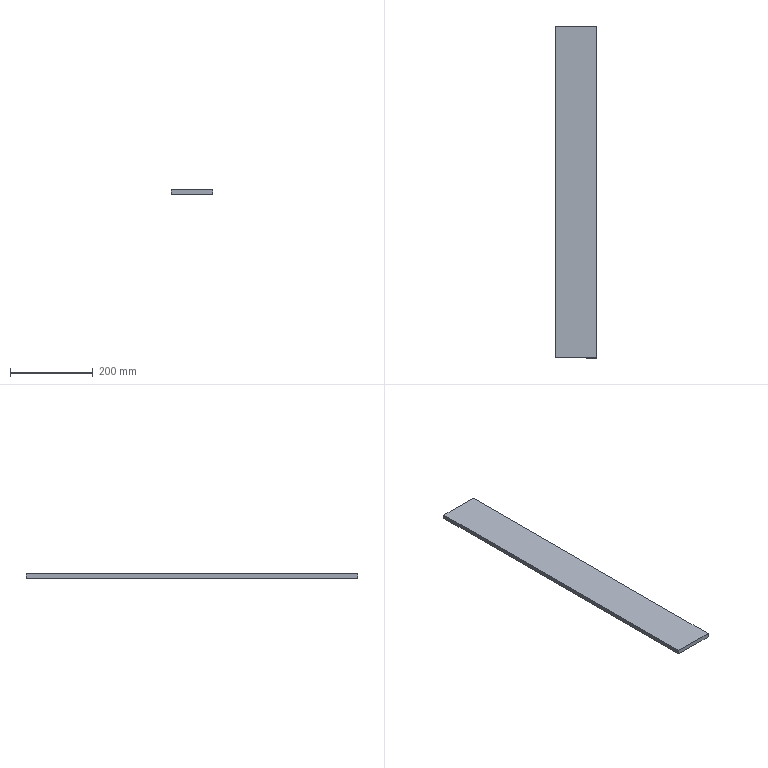Part | STEP file | C2 | 1 solid | 6 faces | box 100 x 800 x 10 mm | volume 800000 mm3 | plane 6
STEP:
#1=CARTESIAN_POINT('',(0.,0.,0.));
#2=DIRECTION('',(0.,0.,1.));
#3=DIRECTION('',(1.,0.,0.));
#4=AXIS2_PLACEMENT_3D('',#1,#2,#3);
#5=CARTESIAN_POINT('',(0.,800.,0.));
#6=VERTEX_POINT('',#5);
#7=CARTESIAN_POINT('',(0.,0.,0.));
#8=VERTEX_POINT('',#7);
#9=CARTESIAN_POINT('',(0.,800.,0.));
#10=DIRECTION('',(0.,-1.,0.));
#11=VECTOR('',#10,1.);
#12=LINE('',#9,#11);
#13=CARTESIAN_POINT('',(0.,800.,-10.));
#14=DIRECTION('',(-1.,0.,0.));
#15=DIRECTION('',(0.,-1.,0.));
#16=AXIS2_PLACEMENT_3D('',#13,#14,#15);
#17=PLANE('',#16);
#18=CARTESIAN_POINT('',(0.,10.));
#19=DIRECTION('',(1.,0.));
#20=VECTOR('',#19,1.);
#21=LINE('',#18,#20);
#22=(GEOMETRIC_REPRESENTATION_CONTEXT(2)PARAMETRIC_REPRESENTATION_CONTEXT()REPRESENTATION_CONTEXT('',''));
#23=DEFINITIONAL_REPRESENTATION('',(#21),#22);
#24=PCURVE('',#17,#23);
#25=CARTESIAN_POINT('',(0.,0.,0.));
#26=DIRECTION('',(0.,0.,1.));
#27=DIRECTION('',(1.,0.,0.));
#28=AXIS2_PLACEMENT_3D('',#25,#26,#27);
#29=PLANE('',#28);
#30=CARTESIAN_POINT('',(0.,800.));
#31=DIRECTION('',(0.,-1.));
#32=VECTOR('',#31,1.);
#33=LINE('',#30,#32);
#34=(GEOMETRIC_REPRESENTATION_CONTEXT(2)PARAMETRIC_REPRESENTATION_CONTEXT()REPRESENTATION_CONTEXT('',''));
#35=DEFINITIONAL_REPRESENTATION('',(#33),#34);
#36=PCURVE('',#29,#35);
#37=SURFACE_CURVE('',#12,(#24,#36),.PCURVE_S1.);
#38=EDGE_CURVE('',#6,#8,#37,.T.);
#39=ORIENTED_EDGE('',*,*,#38,.F.);
#40=CARTESIAN_POINT('',(0.,800.,-10.));
#41=VERTEX_POINT('',#40);
#42=CARTESIAN_POINT('',(0.,800.,-10.));
#43=DIRECTION('',(0.,0.,1.));
#44=VECTOR('',#43,1.);
#45=LINE('',#42,#44);
#46=CARTESIAN_POINT('',(0.,0.));
#47=DIRECTION('',(0.,1.));
#48=VECTOR('',#47,1.);
#49=LINE('',#46,#48);
#50=(GEOMETRIC_REPRESENTATION_CONTEXT(2)PARAMETRIC_REPRESENTATION_CONTEXT()REPRESENTATION_CONTEXT('',''));
#51=DEFINITIONAL_REPRESENTATION('',(#49),#50);
#52=PCURVE('',#17,#51);
#53=CARTESIAN_POINT('',(0.,800.,-10.));
#54=DIRECTION('',(0.,1.,0.));
#55=DIRECTION('',(-1.,0.,0.));
#56=AXIS2_PLACEMENT_3D('',#53,#54,#55);
#57=PLANE('',#56);
#58=CARTESIAN_POINT('',(0.,0.));
#59=DIRECTION('',(0.,1.));
#60=VECTOR('',#59,1.);
#61=LINE('',#58,#60);
#62=(GEOMETRIC_REPRESENTATION_CONTEXT(2)PARAMETRIC_REPRESENTATION_CONTEXT()REPRESENTATION_CONTEXT('',''));
#63=DEFINITIONAL_REPRESENTATION('',(#61),#62);
#64=PCURVE('',#57,#63);
#65=SURFACE_CURVE('',#45,(#52,#64),.PCURVE_S1.);
#66=EDGE_CURVE('',#41,#6,#65,.T.);
#67=ORIENTED_EDGE('',*,*,#66,.F.);
#68=CARTESIAN_POINT('',(0.,0.,-10.));
#69=VERTEX_POINT('',#68);
#70=CARTESIAN_POINT('',(0.,800.,-10.));
#71=DIRECTION('',(0.,-1.,0.));
#72=VECTOR('',#71,1.);
#73=LINE('',#70,#72);
#74=CARTESIAN_POINT('',(0.,0.));
#75=DIRECTION('',(1.,0.));
#76=VECTOR('',#75,1.);
#77=LINE('',#74,#76);
#78=(GEOMETRIC_REPRESENTATION_CONTEXT(2)PARAMETRIC_REPRESENTATION_CONTEXT()REPRESENTATION_CONTEXT('',''));
#79=DEFINITIONAL_REPRESENTATION('',(#77),#78);
#80=PCURVE('',#17,#79);
#81=CARTESIAN_POINT('',(0.,0.,-10.));
#82=DIRECTION('',(0.,0.,1.));
#83=DIRECTION('',(1.,0.,0.));
#84=AXIS2_PLACEMENT_3D('',#81,#82,#83);
#85=PLANE('',#84);
#86=CARTESIAN_POINT('',(0.,800.));
#87=DIRECTION('',(0.,-1.));
#88=VECTOR('',#87,1.);
#89=LINE('',#86,#88);
#90=(GEOMETRIC_REPRESENTATION_CONTEXT(2)PARAMETRIC_REPRESENTATION_CONTEXT()REPRESENTATION_CONTEXT('',''));
#91=DEFINITIONAL_REPRESENTATION('',(#89),#90);
#92=PCURVE('',#85,#91);
#93=SURFACE_CURVE('',#73,(#80,#92),.PCURVE_S1.);
#94=EDGE_CURVE('',#41,#69,#93,.T.);
#95=ORIENTED_EDGE('',*,*,#94,.T.);
#96=CARTESIAN_POINT('',(0.,0.,-10.));
#97=DIRECTION('',(0.,0.,1.));
#98=VECTOR('',#97,1.);
#99=LINE('',#96,#98);
#100=CARTESIAN_POINT('',(800.,0.));
#101=DIRECTION('',(0.,1.));
#102=VECTOR('',#101,1.);
#103=LINE('',#100,#102);
#104=(GEOMETRIC_REPRESENTATION_CONTEXT(2)PARAMETRIC_REPRESENTATION_CONTEXT()REPRESENTATION_CONTEXT('',''));
#105=DEFINITIONAL_REPRESENTATION('',(#103),#104);
#106=PCURVE('',#17,#105);
#107=CARTESIAN_POINT('',(0.,0.,-10.));
#108=DIRECTION('',(0.,-1.,0.));
#109=DIRECTION('',(1.,0.,0.));
#110=AXIS2_PLACEMENT_3D('',#107,#108,#109);
#111=PLANE('',#110);
#112=CARTESIAN_POINT('',(0.,0.));
#113=DIRECTION('',(0.,1.));
#114=VECTOR('',#113,1.);
#115=LINE('',#112,#114);
#116=(GEOMETRIC_REPRESENTATION_CONTEXT(2)PARAMETRIC_REPRESENTATION_CONTEXT()REPRESENTATION_CONTEXT('',''));
#117=DEFINITIONAL_REPRESENTATION('',(#115),#116);
#118=PCURVE('',#111,#117);
#119=SURFACE_CURVE('',#99,(#106,#118),.PCURVE_S1.);
#120=EDGE_CURVE('',#69,#8,#119,.T.);
#121=ORIENTED_EDGE('',*,*,#120,.T.);
#122=EDGE_LOOP('',(#39,#67,#95,#121));
#123=FACE_BOUND('',#122,.T.);
#124=ADVANCED_FACE('',(#123),#17,.T.);
#125=CARTESIAN_POINT('',(100.,800.,0.));
#126=VERTEX_POINT('',#125);
#127=CARTESIAN_POINT('',(0.,800.,0.));
#128=DIRECTION('',(-1.,0.,0.));
#129=VECTOR('',#128,1.);
#130=LINE('',#127,#129);
#131=CARTESIAN_POINT('',(0.,10.));
#132=DIRECTION('',(1.,0.));
#133=VECTOR('',#132,1.);
#134=LINE('',#131,#133);
#135=(GEOMETRIC_REPRESENTATION_CONTEXT(2)PARAMETRIC_REPRESENTATION_CONTEXT()REPRESENTATION_CONTEXT('',''));
#136=DEFINITIONAL_REPRESENTATION('',(#134),#135);
#137=PCURVE('',#57,#136);
#138=CARTESIAN_POINT('',(0.,800.));
#139=DIRECTION('',(-1.,0.));
#140=VECTOR('',#139,1.);
#141=LINE('',#138,#140);
#142=(GEOMETRIC_REPRESENTATION_CONTEXT(2)PARAMETRIC_REPRESENTATION_CONTEXT()REPRESENTATION_CONTEXT('',''));
#143=DEFINITIONAL_REPRESENTATION('',(#141),#142);
#144=PCURVE('',#29,#143);
#145=SURFACE_CURVE('',#130,(#137,#144),.PCURVE_S1.);
#146=EDGE_CURVE('',#126,#6,#145,.T.);
#147=ORIENTED_EDGE('',*,*,#146,.F.);
#148=CARTESIAN_POINT('',(100.,800.,-10.));
#149=VERTEX_POINT('',#148);
#150=CARTESIAN_POINT('',(100.,800.,-10.));
#151=DIRECTION('',(0.,0.,1.));
#152=VECTOR('',#151,1.);
#153=LINE('',#150,#152);
#154=CARTESIAN_POINT('',(-100.,0.));
#155=DIRECTION('',(0.,1.));
#156=VECTOR('',#155,1.);
#157=LINE('',#154,#156);
#158=(GEOMETRIC_REPRESENTATION_CONTEXT(2)PARAMETRIC_REPRESENTATION_CONTEXT()REPRESENTATION_CONTEXT('',''));
#159=DEFINITIONAL_REPRESENTATION('',(#157),#158);
#160=PCURVE('',#57,#159);
#161=CARTESIAN_POINT('',(100.,800.,-10.));
#162=DIRECTION('',(1.,0.,0.));
#163=DIRECTION('',(0.,1.,0.));
#164=AXIS2_PLACEMENT_3D('',#161,#162,#163);
#165=PLANE('',#164);
#166=CARTESIAN_POINT('',(0.,0.));
#167=DIRECTION('',(0.,1.));
#168=VECTOR('',#167,1.);
#169=LINE('',#166,#168);
#170=(GEOMETRIC_REPRESENTATION_CONTEXT(2)PARAMETRIC_REPRESENTATION_CONTEXT()REPRESENTATION_CONTEXT('',''));
#171=DEFINITIONAL_REPRESENTATION('',(#169),#170);
#172=PCURVE('',#165,#171);
#173=SURFACE_CURVE('',#153,(#160,#172),.PCURVE_S1.);
#174=EDGE_CURVE('',#149,#126,#173,.T.);
#175=ORIENTED_EDGE('',*,*,#174,.F.);
#176=CARTESIAN_POINT('',(0.,800.,-10.));
#177=DIRECTION('',(-1.,0.,0.));
#178=VECTOR('',#177,1.);
#179=LINE('',#176,#178);
#180=CARTESIAN_POINT('',(0.,0.));
#181=DIRECTION('',(1.,0.));
#182=VECTOR('',#181,1.);
#183=LINE('',#180,#182);
#184=(GEOMETRIC_REPRESENTATION_CONTEXT(2)PARAMETRIC_REPRESENTATION_CONTEXT()REPRESENTATION_CONTEXT('',''));
#185=DEFINITIONAL_REPRESENTATION('',(#183),#184);
#186=PCURVE('',#57,#185);
#187=CARTESIAN_POINT('',(0.,800.));
#188=DIRECTION('',(-1.,0.));
#189=VECTOR('',#188,1.);
#190=LINE('',#187,#189);
#191=(GEOMETRIC_REPRESENTATION_CONTEXT(2)PARAMETRIC_REPRESENTATION_CONTEXT()REPRESENTATION_CONTEXT('',''));
#192=DEFINITIONAL_REPRESENTATION('',(#190),#191);
#193=PCURVE('',#85,#192);
#194=SURFACE_CURVE('',#179,(#186,#193),.PCURVE_S1.);
#195=EDGE_CURVE('',#149,#41,#194,.T.);
#196=ORIENTED_EDGE('',*,*,#195,.T.);
#197=ORIENTED_EDGE('',*,*,#66,.T.);
#198=EDGE_LOOP('',(#147,#175,#196,#197));
#199=FACE_BOUND('',#198,.T.);
#200=ADVANCED_FACE('',(#199),#57,.T.);
#201=CARTESIAN_POINT('',(100.,0.,0.));
#202=VERTEX_POINT('',#201);
#203=CARTESIAN_POINT('',(100.,800.,0.));
#204=DIRECTION('',(0.,1.,0.));
#205=VECTOR('',#204,1.);
#206=LINE('',#203,#205);
#207=CARTESIAN_POINT('',(0.,10.));
#208=DIRECTION('',(1.,0.));
#209=VECTOR('',#208,1.);
#210=LINE('',#207,#209);
#211=(GEOMETRIC_REPRESENTATION_CONTEXT(2)PARAMETRIC_REPRESENTATION_CONTEXT()REPRESENTATION_CONTEXT('',''));
#212=DEFINITIONAL_REPRESENTATION('',(#210),#211);
#213=PCURVE('',#165,#212);
#214=CARTESIAN_POINT('',(100.,800.));
#215=DIRECTION('',(0.,1.));
#216=VECTOR('',#215,1.);
#217=LINE('',#214,#216);
#218=(GEOMETRIC_REPRESENTATION_CONTEXT(2)PARAMETRIC_REPRESENTATION_CONTEXT()REPRESENTATION_CONTEXT('',''));
#219=DEFINITIONAL_REPRESENTATION('',(#217),#218);
#220=PCURVE('',#29,#219);
#221=SURFACE_CURVE('',#206,(#213,#220),.PCURVE_S1.);
#222=EDGE_CURVE('',#202,#126,#221,.T.);
#223=ORIENTED_EDGE('',*,*,#222,.F.);
#224=CARTESIAN_POINT('',(100.,0.,-10.));
#225=VERTEX_POINT('',#224);
#226=CARTESIAN_POINT('',(100.,0.,-10.));
#227=DIRECTION('',(0.,0.,1.));
#228=VECTOR('',#227,1.);
#229=LINE('',#226,#228);
#230=CARTESIAN_POINT('',(-800.,0.));
#231=DIRECTION('',(0.,1.));
#232=VECTOR('',#231,1.);
#233=LINE('',#230,#232);
#234=(GEOMETRIC_REPRESENTATION_CONTEXT(2)PARAMETRIC_REPRESENTATION_CONTEXT()REPRESENTATION_CONTEXT('',''));
#235=DEFINITIONAL_REPRESENTATION('',(#233),#234);
#236=PCURVE('',#165,#235);
#237=CARTESIAN_POINT('',(100.,0.));
#238=DIRECTION('',(0.,1.));
#239=VECTOR('',#238,1.);
#240=LINE('',#237,#239);
#241=(GEOMETRIC_REPRESENTATION_CONTEXT(2)PARAMETRIC_REPRESENTATION_CONTEXT()REPRESENTATION_CONTEXT('',''));
#242=DEFINITIONAL_REPRESENTATION('',(#240),#241);
#243=PCURVE('',#111,#242);
#244=SURFACE_CURVE('',#229,(#236,#243),.PCURVE_S1.);
#245=EDGE_CURVE('',#225,#202,#244,.T.);
#246=ORIENTED_EDGE('',*,*,#245,.F.);
#247=CARTESIAN_POINT('',(100.,800.,-10.));
#248=DIRECTION('',(0.,1.,0.));
#249=VECTOR('',#248,1.);
#250=LINE('',#247,#249);
#251=CARTESIAN_POINT('',(0.,0.));
#252=DIRECTION('',(1.,0.));
#253=VECTOR('',#252,1.);
#254=LINE('',#251,#253);
#255=(GEOMETRIC_REPRESENTATION_CONTEXT(2)PARAMETRIC_REPRESENTATION_CONTEXT()REPRESENTATION_CONTEXT('',''));
#256=DEFINITIONAL_REPRESENTATION('',(#254),#255);
#257=PCURVE('',#165,#256);
#258=CARTESIAN_POINT('',(100.,800.));
#259=DIRECTION('',(0.,1.));
#260=VECTOR('',#259,1.);
#261=LINE('',#258,#260);
#262=(GEOMETRIC_REPRESENTATION_CONTEXT(2)PARAMETRIC_REPRESENTATION_CONTEXT()REPRESENTATION_CONTEXT('',''));
#263=DEFINITIONAL_REPRESENTATION('',(#261),#262);
#264=PCURVE('',#85,#263);
#265=SURFACE_CURVE('',#250,(#257,#264),.PCURVE_S1.);
#266=EDGE_CURVE('',#225,#149,#265,.T.);
#267=ORIENTED_EDGE('',*,*,#266,.T.);
#268=ORIENTED_EDGE('',*,*,#174,.T.);
#269=EDGE_LOOP('',(#223,#246,#267,#268));
#270=FACE_BOUND('',#269,.T.);
#271=ADVANCED_FACE('',(#270),#165,.T.);
#272=CARTESIAN_POINT('',(0.,0.,0.));
#273=DIRECTION('',(1.,0.,0.));
#274=VECTOR('',#273,1.);
#275=LINE('',#272,#274);
#276=CARTESIAN_POINT('',(0.,10.));
#277=DIRECTION('',(1.,0.));
#278=VECTOR('',#277,1.);
#279=LINE('',#276,#278);
#280=(GEOMETRIC_REPRESENTATION_CONTEXT(2)PARAMETRIC_REPRESENTATION_CONTEXT()REPRESENTATION_CONTEXT('',''));
#281=DEFINITIONAL_REPRESENTATION('',(#279),#280);
#282=PCURVE('',#111,#281);
#283=CARTESIAN_POINT('',(0.,0.));
#284=DIRECTION('',(1.,0.));
#285=VECTOR('',#284,1.);
#286=LINE('',#283,#285);
#287=(GEOMETRIC_REPRESENTATION_CONTEXT(2)PARAMETRIC_REPRESENTATION_CONTEXT()REPRESENTATION_CONTEXT('',''));
#288=DEFINITIONAL_REPRESENTATION('',(#286),#287);
#289=PCURVE('',#29,#288);
#290=SURFACE_CURVE('',#275,(#282,#289),.PCURVE_S1.);
#291=EDGE_CURVE('',#8,#202,#290,.T.);
#292=ORIENTED_EDGE('',*,*,#291,.F.);
#293=ORIENTED_EDGE('',*,*,#120,.F.);
#294=CARTESIAN_POINT('',(0.,0.,-10.));
#295=DIRECTION('',(1.,0.,0.));
#296=VECTOR('',#295,1.);
#297=LINE('',#294,#296);
#298=CARTESIAN_POINT('',(0.,0.));
#299=DIRECTION('',(1.,0.));
#300=VECTOR('',#299,1.);
#301=LINE('',#298,#300);
#302=(GEOMETRIC_REPRESENTATION_CONTEXT(2)PARAMETRIC_REPRESENTATION_CONTEXT()REPRESENTATION_CONTEXT('',''));
#303=DEFINITIONAL_REPRESENTATION('',(#301),#302);
#304=PCURVE('',#111,#303);
#305=CARTESIAN_POINT('',(0.,0.));
#306=DIRECTION('',(1.,0.));
#307=VECTOR('',#306,1.);
#308=LINE('',#305,#307);
#309=(GEOMETRIC_REPRESENTATION_CONTEXT(2)PARAMETRIC_REPRESENTATION_CONTEXT()REPRESENTATION_CONTEXT('',''));
#310=DEFINITIONAL_REPRESENTATION('',(#308),#309);
#311=PCURVE('',#85,#310);
#312=SURFACE_CURVE('',#297,(#304,#311),.PCURVE_S1.);
#313=EDGE_CURVE('',#69,#225,#312,.T.);
#314=ORIENTED_EDGE('',*,*,#313,.T.);
#315=ORIENTED_EDGE('',*,*,#245,.T.);
#316=EDGE_LOOP('',(#292,#293,#314,#315));
#317=FACE_BOUND('',#316,.T.);
#318=ADVANCED_FACE('',(#317),#111,.T.);
#319=ORIENTED_EDGE('',*,*,#94,.F.);
#320=ORIENTED_EDGE('',*,*,#195,.F.);
#321=ORIENTED_EDGE('',*,*,#266,.F.);
#322=ORIENTED_EDGE('',*,*,#313,.F.);
#323=EDGE_LOOP('',(#319,#320,#321,#322));
#324=FACE_BOUND('',#323,.T.);
#325=ADVANCED_FACE('',(#324),#85,.F.);
#326=ORIENTED_EDGE('',*,*,#38,.T.);
#327=ORIENTED_EDGE('',*,*,#291,.T.);
#328=ORIENTED_EDGE('',*,*,#222,.T.);
#329=ORIENTED_EDGE('',*,*,#146,.T.);
#330=EDGE_LOOP('',(#326,#327,#328,#329));
#331=FACE_BOUND('',#330,.T.);
#332=ADVANCED_FACE('',(#331),#29,.T.);
#333=CLOSED_SHELL('',(#124,#200,#271,#318,#325,#332));
#334=MANIFOLD_SOLID_BREP('',#333);
#335=(LENGTH_UNIT()NAMED_UNIT(*)SI_UNIT(.MILLI.,.METRE.));
#336=UNCERTAINTY_MEASURE_WITH_UNIT(LENGTH_MEASURE(0.0000001),#335,'','');
#337=(NAMED_UNIT(*)PLANE_ANGLE_UNIT()SI_UNIT($,.RADIAN.));
#338=(NAMED_UNIT(*)SI_UNIT($,.STERADIAN.)SOLID_ANGLE_UNIT());
#339=(GEOMETRIC_REPRESENTATION_CONTEXT(3)GLOBAL_UNCERTAINTY_ASSIGNED_CONTEXT((#336))GLOBAL_UNIT_ASSIGNED_CONTEXT((#335,#337,#338))REPRESENTATION_CONTEXT('',''));
#340=ADVANCED_BREP_SHAPE_REPRESENTATION('',(#4,#334),#339);